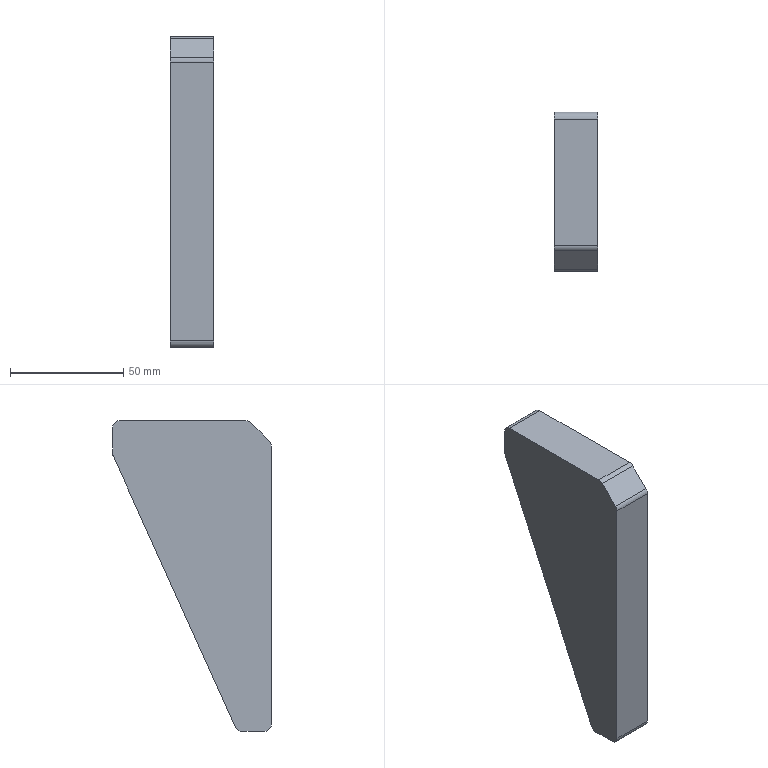Part | STEP file | SN10_010_005-03_REFORCO | 1 solid | 14 faces | box 19 x 70 x 137 mm | volume 117421 mm3 | plane 8 | cylinder 6 | commonest cylinder face diameters 6 x6
STEP:
#1=CARTESIAN_POINT('',(0.,0.,0.));
#2=DIRECTION('',(0.,0.,1.));
#3=DIRECTION('',(1.,0.,0.));
#4=AXIS2_PLACEMENT_3D('',#1,#2,#3);
#5=CARTESIAN_POINT('',(106.,-333.,340.));
#6=VERTEX_POINT('',#5);
#7=CARTESIAN_POINT('',(106.,-330.,337.));
#8=VERTEX_POINT('',#7);
#9=CARTESIAN_POINT('',(106.,-333.,337.));
#10=DIRECTION('',(-1.,0.,0.));
#11=DIRECTION('',(0.,1.,0.));
#12=AXIS2_PLACEMENT_3D('',#9,#10,#11);
#13=CIRCLE('',#12,3.);
#14=CARTESIAN_POINT('',(115.5,-333.,337.));
#15=DIRECTION('',(-1.,0.,0.));
#16=DIRECTION('',(0.,0.,1.));
#17=AXIS2_PLACEMENT_3D('',#14,#15,#16);
#18=CYLINDRICAL_SURFACE('',#17,3.);
#19=CARTESIAN_POINT('',(-4.712,9.5));
#20=DIRECTION('',(1.,0.));
#21=VECTOR('',#20,1.);
#22=LINE('',#19,#21);
#23=(GEOMETRIC_REPRESENTATION_CONTEXT(2)PARAMETRIC_REPRESENTATION_CONTEXT()REPRESENTATION_CONTEXT('',''));
#24=DEFINITIONAL_REPRESENTATION('',(#22),#23);
#25=PCURVE('',#18,#24);
#26=CARTESIAN_POINT('',(106.,0.,0.));
#27=DIRECTION('',(1.,0.,0.));
#28=DIRECTION('',(0.,0.,-1.));
#29=AXIS2_PLACEMENT_3D('',#26,#27,#28);
#30=PLANE('',#29);
#31=CARTESIAN_POINT('',(-337.,-330.));
#32=CARTESIAN_POINT('',(-331.804,-330.));
#33=CARTESIAN_POINT('',(-334.402,-334.5));
#34=CARTESIAN_POINT('',(-337.,-339.));
#35=CARTESIAN_POINT('',(-339.598,-334.5));
#36=CARTESIAN_POINT('',(-342.196,-330.));
#37=CARTESIAN_POINT('',(-337.,-330.));
#38=(BOUNDED_CURVE()B_SPLINE_CURVE(2,(#31,#32,#33,#34,#35,#36,#37),.UNSPECIFIED.,.T.,.F.)B_SPLINE_CURVE_WITH_KNOTS((1,2,2,2,2,1),(-2.094,0.,2.094,4.189,6.283,8.378),.UNSPECIFIED.)CURVE()GEOMETRIC_REPRESENTATION_ITEM()RATIONAL_B_SPLINE_CURVE((1.,0.5,1.,0.5,1.,0.5,1.))REPRESENTATION_ITEM(''));
#39=(GEOMETRIC_REPRESENTATION_CONTEXT(2)PARAMETRIC_REPRESENTATION_CONTEXT()REPRESENTATION_CONTEXT('',''));
#40=DEFINITIONAL_REPRESENTATION('',(#38),#39);
#41=PCURVE('',#30,#40);
#42=SURFACE_CURVE('',#13,(#25,#41),.PCURVE_S1.);
#43=EDGE_CURVE('',#6,#8,#42,.T.);
#44=ORIENTED_EDGE('',*,*,#43,.F.);
#45=CARTESIAN_POINT('',(125.,-333.,340.));
#46=VERTEX_POINT('',#45);
#47=CARTESIAN_POINT('',(125.,-333.,340.));
#48=DIRECTION('',(-1.,0.,0.));
#49=VECTOR('',#48,1.);
#50=LINE('',#47,#49);
#51=CARTESIAN_POINT('',(0.,-9.5));
#52=DIRECTION('',(0.,1.));
#53=VECTOR('',#52,1.);
#54=LINE('',#51,#53);
#55=(GEOMETRIC_REPRESENTATION_CONTEXT(2)PARAMETRIC_REPRESENTATION_CONTEXT()REPRESENTATION_CONTEXT('',''));
#56=DEFINITIONAL_REPRESENTATION('',(#54),#55);
#57=PCURVE('',#18,#56);
#58=CARTESIAN_POINT('',(125.,-330.,340.));
#59=DIRECTION('',(0.,0.,-1.));
#60=DIRECTION('',(-1.,0.,0.));
#61=AXIS2_PLACEMENT_3D('',#58,#59,#60);
#62=PLANE('',#61);
#63=CARTESIAN_POINT('',(0.,-3.));
#64=DIRECTION('',(1.,0.));
#65=VECTOR('',#64,1.);
#66=LINE('',#63,#65);
#67=(GEOMETRIC_REPRESENTATION_CONTEXT(2)PARAMETRIC_REPRESENTATION_CONTEXT()REPRESENTATION_CONTEXT('',''));
#68=DEFINITIONAL_REPRESENTATION('',(#66),#67);
#69=PCURVE('',#62,#68);
#70=SURFACE_CURVE('',#50,(#57,#69),.PCURVE_S1.);
#71=EDGE_CURVE('',#46,#6,#70,.T.);
#72=ORIENTED_EDGE('',*,*,#71,.F.);
#73=CARTESIAN_POINT('',(125.,-330.,337.));
#74=VERTEX_POINT('',#73);
#75=CARTESIAN_POINT('',(125.,-333.,337.));
#76=DIRECTION('',(-1.,0.,0.));
#77=DIRECTION('',(0.,1.,0.));
#78=AXIS2_PLACEMENT_3D('',#75,#76,#77);
#79=CIRCLE('',#78,3.);
#80=CARTESIAN_POINT('',(-4.712,-9.5));
#81=DIRECTION('',(1.,0.));
#82=VECTOR('',#81,1.);
#83=LINE('',#80,#82);
#84=(GEOMETRIC_REPRESENTATION_CONTEXT(2)PARAMETRIC_REPRESENTATION_CONTEXT()REPRESENTATION_CONTEXT('',''));
#85=DEFINITIONAL_REPRESENTATION('',(#83),#84);
#86=PCURVE('',#18,#85);
#87=CARTESIAN_POINT('',(125.,0.,0.));
#88=DIRECTION('',(1.,0.,0.));
#89=DIRECTION('',(0.,0.,-1.));
#90=AXIS2_PLACEMENT_3D('',#87,#88,#89);
#91=PLANE('',#90);
#92=CARTESIAN_POINT('',(-337.,-330.));
#93=CARTESIAN_POINT('',(-331.804,-330.));
#94=CARTESIAN_POINT('',(-334.402,-334.5));
#95=CARTESIAN_POINT('',(-337.,-339.));
#96=CARTESIAN_POINT('',(-339.598,-334.5));
#97=CARTESIAN_POINT('',(-342.196,-330.));
#98=CARTESIAN_POINT('',(-337.,-330.));
#99=(BOUNDED_CURVE()B_SPLINE_CURVE(2,(#92,#93,#94,#95,#96,#97,#98),.UNSPECIFIED.,.T.,.F.)B_SPLINE_CURVE_WITH_KNOTS((1,2,2,2,2,1),(-2.094,0.,2.094,4.189,6.283,8.378),.UNSPECIFIED.)CURVE()GEOMETRIC_REPRESENTATION_ITEM()RATIONAL_B_SPLINE_CURVE((1.,0.5,1.,0.5,1.,0.5,1.))REPRESENTATION_ITEM(''));
#100=(GEOMETRIC_REPRESENTATION_CONTEXT(2)PARAMETRIC_REPRESENTATION_CONTEXT()REPRESENTATION_CONTEXT('',''));
#101=DEFINITIONAL_REPRESENTATION('',(#99),#100);
#102=PCURVE('',#91,#101);
#103=SURFACE_CURVE('',#79,(#86,#102),.PCURVE_S1.);
#104=EDGE_CURVE('',#46,#74,#103,.T.);
#105=ORIENTED_EDGE('',*,*,#104,.T.);
#106=CARTESIAN_POINT('',(125.,-330.,337.));
#107=DIRECTION('',(-1.,0.,0.));
#108=VECTOR('',#107,1.);
#109=LINE('',#106,#108);
#110=CARTESIAN_POINT('',(1.571,-9.5));
#111=DIRECTION('',(0.,1.));
#112=VECTOR('',#111,1.);
#113=LINE('',#110,#112);
#114=(GEOMETRIC_REPRESENTATION_CONTEXT(2)PARAMETRIC_REPRESENTATION_CONTEXT()REPRESENTATION_CONTEXT('',''));
#115=DEFINITIONAL_REPRESENTATION('',(#113),#114);
#116=PCURVE('',#18,#115);
#117=CARTESIAN_POINT('',(125.,-330.,325.));
#118=DIRECTION('',(0.,-1.,0.));
#119=DIRECTION('',(0.,0.,-1.));
#120=AXIS2_PLACEMENT_3D('',#117,#118,#119);
#121=PLANE('',#120);
#122=CARTESIAN_POINT('',(-12.,0.));
#123=DIRECTION('',(0.,-1.));
#124=VECTOR('',#123,1.);
#125=LINE('',#122,#124);
#126=(GEOMETRIC_REPRESENTATION_CONTEXT(2)PARAMETRIC_REPRESENTATION_CONTEXT()REPRESENTATION_CONTEXT('',''));
#127=DEFINITIONAL_REPRESENTATION('',(#125),#126);
#128=PCURVE('',#121,#127);
#129=SURFACE_CURVE('',#109,(#116,#128),.PCURVE_S1.);
#130=EDGE_CURVE('',#74,#8,#129,.T.);
#131=ORIENTED_EDGE('',*,*,#130,.T.);
#132=EDGE_LOOP('',(#44,#72,#105,#131));
#133=FACE_BOUND('',#132,.T.);
#134=ADVANCED_FACE('',(#133),#18,.T.);
#135=CARTESIAN_POINT('',(125.,-330.,325.645));
#136=VERTEX_POINT('',#135);
#137=CARTESIAN_POINT('',(106.,-330.,325.645));
#138=VERTEX_POINT('',#137);
#139=CARTESIAN_POINT('',(125.,-330.,325.645));
#140=DIRECTION('',(-1.,0.,0.));
#141=VECTOR('',#140,1.);
#142=LINE('',#139,#141);
#143=CARTESIAN_POINT('',(-0.645,0.));
#144=DIRECTION('',(0.,-1.));
#145=VECTOR('',#144,1.);
#146=LINE('',#143,#145);
#147=(GEOMETRIC_REPRESENTATION_CONTEXT(2)PARAMETRIC_REPRESENTATION_CONTEXT()REPRESENTATION_CONTEXT('',''));
#148=DEFINITIONAL_REPRESENTATION('',(#146),#147);
#149=PCURVE('',#121,#148);
#150=CARTESIAN_POINT('',(115.5,-333.,325.645));
#151=DIRECTION('',(-1.,0.,0.));
#152=DIRECTION('',(0.,1.,0.));
#153=AXIS2_PLACEMENT_3D('',#150,#151,#152);
#154=CYLINDRICAL_SURFACE('',#153,3.);
#155=CARTESIAN_POINT('',(0.,-9.5));
#156=DIRECTION('',(0.,1.));
#157=VECTOR('',#156,1.);
#158=LINE('',#155,#157);
#159=(GEOMETRIC_REPRESENTATION_CONTEXT(2)PARAMETRIC_REPRESENTATION_CONTEXT()REPRESENTATION_CONTEXT('',''));
#160=DEFINITIONAL_REPRESENTATION('',(#158),#159);
#161=PCURVE('',#154,#160);
#162=SURFACE_CURVE('',#142,(#149,#161),.PCURVE_S1.);
#163=EDGE_CURVE('',#136,#138,#162,.T.);
#164=ORIENTED_EDGE('',*,*,#163,.T.);
#165=CARTESIAN_POINT('',(106.,-330.,325.645));
#166=DIRECTION('',(0.,0.,1.));
#167=VECTOR('',#166,1.);
#168=LINE('',#165,#167);
#169=CARTESIAN_POINT('',(-0.645,-19.));
#170=DIRECTION('',(-1.,0.));
#171=VECTOR('',#170,1.);
#172=LINE('',#169,#171);
#173=(GEOMETRIC_REPRESENTATION_CONTEXT(2)PARAMETRIC_REPRESENTATION_CONTEXT()REPRESENTATION_CONTEXT('',''));
#174=DEFINITIONAL_REPRESENTATION('',(#172),#173);
#175=PCURVE('',#121,#174);
#176=CARTESIAN_POINT('',(-325.645,-330.));
#177=DIRECTION('',(-1.,0.));
#178=VECTOR('',#177,1.);
#179=LINE('',#176,#178);
#180=(GEOMETRIC_REPRESENTATION_CONTEXT(2)PARAMETRIC_REPRESENTATION_CONTEXT()REPRESENTATION_CONTEXT('',''));
#181=DEFINITIONAL_REPRESENTATION('',(#179),#180);
#182=PCURVE('',#30,#181);
#183=SURFACE_CURVE('',#168,(#175,#182),.PCURVE_S1.);
#184=EDGE_CURVE('',#138,#8,#183,.T.);
#185=ORIENTED_EDGE('',*,*,#184,.T.);
#186=ORIENTED_EDGE('',*,*,#130,.F.);
#187=CARTESIAN_POINT('',(125.,-330.,325.645));
#188=DIRECTION('',(0.,0.,1.));
#189=VECTOR('',#188,1.);
#190=LINE('',#187,#189);
#191=CARTESIAN_POINT('',(-0.645,0.));
#192=DIRECTION('',(-1.,0.));
#193=VECTOR('',#192,1.);
#194=LINE('',#191,#193);
#195=(GEOMETRIC_REPRESENTATION_CONTEXT(2)PARAMETRIC_REPRESENTATION_CONTEXT()REPRESENTATION_CONTEXT('',''));
#196=DEFINITIONAL_REPRESENTATION('',(#194),#195);
#197=PCURVE('',#121,#196);
#198=CARTESIAN_POINT('',(-325.645,-330.));
#199=DIRECTION('',(-1.,0.));
#200=VECTOR('',#199,1.);
#201=LINE('',#198,#200);
#202=(GEOMETRIC_REPRESENTATION_CONTEXT(2)PARAMETRIC_REPRESENTATION_CONTEXT()REPRESENTATION_CONTEXT('',''));
#203=DEFINITIONAL_REPRESENTATION('',(#201),#202);
#204=PCURVE('',#91,#203);
#205=SURFACE_CURVE('',#190,(#197,#204),.PCURVE_S1.);
#206=EDGE_CURVE('',#136,#74,#205,.T.);
#207=ORIENTED_EDGE('',*,*,#206,.F.);
#208=EDGE_LOOP('',(#164,#185,#186,#207));
#209=FACE_BOUND('',#208,.T.);
#210=ADVANCED_FACE('',(#209),#121,.F.);
#211=CARTESIAN_POINT('',(106.,-330.265,324.412));
#212=VERTEX_POINT('',#211);
#213=CARTESIAN_POINT('',(106.,-333.,325.645));
#214=DIRECTION('',(-1.,0.,0.));
#215=DIRECTION('',(0.,1.,0.));
#216=AXIS2_PLACEMENT_3D('',#213,#214,#215);
#217=CIRCLE('',#216,3.);
#218=CARTESIAN_POINT('',(0.,9.5));
#219=DIRECTION('',(1.,0.));
#220=VECTOR('',#219,1.);
#221=LINE('',#218,#220);
#222=(GEOMETRIC_REPRESENTATION_CONTEXT(2)PARAMETRIC_REPRESENTATION_CONTEXT()REPRESENTATION_CONTEXT('',''));
#223=DEFINITIONAL_REPRESENTATION('',(#221),#222);
#224=PCURVE('',#154,#223);
#225=CARTESIAN_POINT('',(-325.645,-330.));
#226=CARTESIAN_POINT('',(-320.449,-330.));
#227=CARTESIAN_POINT('',(-323.047,-334.5));
#228=CARTESIAN_POINT('',(-325.645,-339.));
#229=CARTESIAN_POINT('',(-328.243,-334.5));
#230=CARTESIAN_POINT('',(-330.841,-330.));
#231=CARTESIAN_POINT('',(-325.645,-330.));
#232=(BOUNDED_CURVE()B_SPLINE_CURVE(2,(#225,#226,#227,#228,#229,#230,#231),.UNSPECIFIED.,.T.,.F.)B_SPLINE_CURVE_WITH_KNOTS((1,2,2,2,2,1),(-2.094,0.,2.094,4.189,6.283,8.378),.UNSPECIFIED.)CURVE()GEOMETRIC_REPRESENTATION_ITEM()RATIONAL_B_SPLINE_CURVE((1.,0.5,1.,0.5,1.,0.5,1.))REPRESENTATION_ITEM(''));
#233=(GEOMETRIC_REPRESENTATION_CONTEXT(2)PARAMETRIC_REPRESENTATION_CONTEXT()REPRESENTATION_CONTEXT('',''));
#234=DEFINITIONAL_REPRESENTATION('',(#232),#233);
#235=PCURVE('',#30,#234);
#236=SURFACE_CURVE('',#217,(#224,#235),.PCURVE_S1.);
#237=EDGE_CURVE('',#138,#212,#236,.T.);
#238=ORIENTED_EDGE('',*,*,#237,.F.);
#239=ORIENTED_EDGE('',*,*,#163,.F.);
#240=CARTESIAN_POINT('',(125.,-330.265,324.412));
#241=VERTEX_POINT('',#240);
#242=CARTESIAN_POINT('',(125.,-333.,325.645));
#243=DIRECTION('',(-1.,0.,0.));
#244=DIRECTION('',(0.,1.,0.));
#245=AXIS2_PLACEMENT_3D('',#242,#243,#244);
#246=CIRCLE('',#245,3.);
#247=CARTESIAN_POINT('',(0.,-9.5));
#248=DIRECTION('',(1.,0.));
#249=VECTOR('',#248,1.);
#250=LINE('',#247,#249);
#251=(GEOMETRIC_REPRESENTATION_CONTEXT(2)PARAMETRIC_REPRESENTATION_CONTEXT()REPRESENTATION_CONTEXT('',''));
#252=DEFINITIONAL_REPRESENTATION('',(#250),#251);
#253=PCURVE('',#154,#252);
#254=CARTESIAN_POINT('',(-325.645,-330.));
#255=CARTESIAN_POINT('',(-320.449,-330.));
#256=CARTESIAN_POINT('',(-323.047,-334.5));
#257=CARTESIAN_POINT('',(-325.645,-339.));
#258=CARTESIAN_POINT('',(-328.243,-334.5));
#259=CARTESIAN_POINT('',(-330.841,-330.));
#260=CARTESIAN_POINT('',(-325.645,-330.));
#261=(BOUNDED_CURVE()B_SPLINE_CURVE(2,(#254,#255,#256,#257,#258,#259,#260),.UNSPECIFIED.,.T.,.F.)B_SPLINE_CURVE_WITH_KNOTS((1,2,2,2,2,1),(-2.094,0.,2.094,4.189,6.283,8.378),.UNSPECIFIED.)CURVE()GEOMETRIC_REPRESENTATION_ITEM()RATIONAL_B_SPLINE_CURVE((1.,0.5,1.,0.5,1.,0.5,1.))REPRESENTATION_ITEM(''));
#262=(GEOMETRIC_REPRESENTATION_CONTEXT(2)PARAMETRIC_REPRESENTATION_CONTEXT()REPRESENTATION_CONTEXT('',''));
#263=DEFINITIONAL_REPRESENTATION('',(#261),#262);
#264=PCURVE('',#91,#263);
#265=SURFACE_CURVE('',#246,(#253,#264),.PCURVE_S1.);
#266=EDGE_CURVE('',#136,#241,#265,.T.);
#267=ORIENTED_EDGE('',*,*,#266,.T.);
#268=CARTESIAN_POINT('',(125.,-330.265,324.412));
#269=DIRECTION('',(-1.,0.,0.));
#270=VECTOR('',#269,1.);
#271=LINE('',#268,#270);
#272=CARTESIAN_POINT('',(0.4235,-9.5));
#273=DIRECTION('',(0.,1.));
#274=VECTOR('',#273,1.);
#275=LINE('',#272,#274);
#276=(GEOMETRIC_REPRESENTATION_CONTEXT(2)PARAMETRIC_REPRESENTATION_CONTEXT()REPRESENTATION_CONTEXT('',''));
#277=DEFINITIONAL_REPRESENTATION('',(#275),#276);
#278=PCURVE('',#154,#277);
#279=CARTESIAN_POINT('',(125.,-385.,203.));
#280=DIRECTION('',(0.,-0.9116,0.411));
#281=DIRECTION('',(0.,-0.411,-0.9116));
#282=AXIS2_PLACEMENT_3D('',#279,#280,#281);
#283=PLANE('',#282);
#284=CARTESIAN_POINT('',(-133.18,0.));
#285=DIRECTION('',(0.,-1.));
#286=VECTOR('',#285,1.);
#287=LINE('',#284,#286);
#288=(GEOMETRIC_REPRESENTATION_CONTEXT(2)PARAMETRIC_REPRESENTATION_CONTEXT()REPRESENTATION_CONTEXT('',''));
#289=DEFINITIONAL_REPRESENTATION('',(#287),#288);
#290=PCURVE('',#283,#289);
#291=SURFACE_CURVE('',#271,(#278,#290),.PCURVE_S1.);
#292=EDGE_CURVE('',#241,#212,#291,.T.);
#293=ORIENTED_EDGE('',*,*,#292,.T.);
#294=EDGE_LOOP('',(#238,#239,#267,#293));
#295=FACE_BOUND('',#294,.T.);
#296=ADVANCED_FACE('',(#295),#154,.T.);
#297=CARTESIAN_POINT('',(125.,-384.203,204.767));
#298=VERTEX_POINT('',#297);
#299=CARTESIAN_POINT('',(106.,-384.203,204.767));
#300=VERTEX_POINT('',#299);
#301=CARTESIAN_POINT('',(125.,-384.203,204.767));
#302=DIRECTION('',(-1.,0.,0.));
#303=VECTOR('',#302,1.);
#304=LINE('',#301,#303);
#305=CARTESIAN_POINT('',(-1.938,0.));
#306=DIRECTION('',(0.,-1.));
#307=VECTOR('',#306,1.);
#308=LINE('',#305,#307);
#309=(GEOMETRIC_REPRESENTATION_CONTEXT(2)PARAMETRIC_REPRESENTATION_CONTEXT()REPRESENTATION_CONTEXT('',''));
#310=DEFINITIONAL_REPRESENTATION('',(#308),#309);
#311=PCURVE('',#283,#310);
#312=CARTESIAN_POINT('',(115.5,-386.938,206.));
#313=DIRECTION('',(-1.,0.,0.));
#314=DIRECTION('',(0.,0.9116,-0.411));
#315=AXIS2_PLACEMENT_3D('',#312,#313,#314);
#316=CYLINDRICAL_SURFACE('',#315,3.);
#317=CARTESIAN_POINT('',(0.,-9.5));
#318=DIRECTION('',(0.,1.));
#319=VECTOR('',#318,1.);
#320=LINE('',#317,#319);
#321=(GEOMETRIC_REPRESENTATION_CONTEXT(2)PARAMETRIC_REPRESENTATION_CONTEXT()REPRESENTATION_CONTEXT('',''));
#322=DEFINITIONAL_REPRESENTATION('',(#320),#321);
#323=PCURVE('',#316,#322);
#324=SURFACE_CURVE('',#304,(#311,#323),.PCURVE_S1.);
#325=EDGE_CURVE('',#298,#300,#324,.T.);
#326=ORIENTED_EDGE('',*,*,#325,.T.);
#327=CARTESIAN_POINT('',(106.,-384.203,204.767));
#328=DIRECTION('',(0.,0.411,0.9116));
#329=VECTOR('',#328,1.);
#330=LINE('',#327,#329);
#331=CARTESIAN_POINT('',(-1.938,-19.));
#332=DIRECTION('',(-1.,0.));
#333=VECTOR('',#332,1.);
#334=LINE('',#331,#333);
#335=(GEOMETRIC_REPRESENTATION_CONTEXT(2)PARAMETRIC_REPRESENTATION_CONTEXT()REPRESENTATION_CONTEXT('',''));
#336=DEFINITIONAL_REPRESENTATION('',(#334),#335);
#337=PCURVE('',#283,#336);
#338=CARTESIAN_POINT('',(-204.767,-384.203));
#339=DIRECTION('',(-0.9116,0.411));
#340=VECTOR('',#339,1.);
#341=LINE('',#338,#340);
#342=(GEOMETRIC_REPRESENTATION_CONTEXT(2)PARAMETRIC_REPRESENTATION_CONTEXT()REPRESENTATION_CONTEXT('',''));
#343=DEFINITIONAL_REPRESENTATION('',(#341),#342);
#344=PCURVE('',#30,#343);
#345=SURFACE_CURVE('',#330,(#337,#344),.PCURVE_S1.);
#346=EDGE_CURVE('',#300,#212,#345,.T.);
#347=ORIENTED_EDGE('',*,*,#346,.T.);
#348=ORIENTED_EDGE('',*,*,#292,.F.);
#349=CARTESIAN_POINT('',(125.,-384.203,204.767));
#350=DIRECTION('',(0.,0.411,0.9116));
#351=VECTOR('',#350,1.);
#352=LINE('',#349,#351);
#353=CARTESIAN_POINT('',(-1.938,0.));
#354=DIRECTION('',(-1.,0.));
#355=VECTOR('',#354,1.);
#356=LINE('',#353,#355);
#357=(GEOMETRIC_REPRESENTATION_CONTEXT(2)PARAMETRIC_REPRESENTATION_CONTEXT()REPRESENTATION_CONTEXT('',''));
#358=DEFINITIONAL_REPRESENTATION('',(#356),#357);
#359=PCURVE('',#283,#358);
#360=CARTESIAN_POINT('',(-204.767,-384.203));
#361=DIRECTION('',(-0.9116,0.411));
#362=VECTOR('',#361,1.);
#363=LINE('',#360,#362);
#364=(GEOMETRIC_REPRESENTATION_CONTEXT(2)PARAMETRIC_REPRESENTATION_CONTEXT()REPRESENTATION_CONTEXT('',''));
#365=DEFINITIONAL_REPRESENTATION('',(#363),#364);
#366=PCURVE('',#91,#365);
#367=SURFACE_CURVE('',#352,(#359,#366),.PCURVE_S1.);
#368=EDGE_CURVE('',#298,#241,#367,.T.);
#369=ORIENTED_EDGE('',*,*,#368,.F.);
#370=EDGE_LOOP('',(#326,#347,#348,#369));
#371=FACE_BOUND('',#370,.T.);
#372=ADVANCED_FACE('',(#371),#283,.F.);
#373=CARTESIAN_POINT('',(106.,-386.938,203.));
#374=VERTEX_POINT('',#373);
#375=CARTESIAN_POINT('',(106.,-386.938,206.));
#376=DIRECTION('',(-1.,0.,0.));
#377=DIRECTION('',(0.,1.,0.));
#378=AXIS2_PLACEMENT_3D('',#375,#376,#377);
#379=CIRCLE('',#378,3.);
#380=CARTESIAN_POINT('',(-0.4235,9.5));
#381=DIRECTION('',(1.,0.));
#382=VECTOR('',#381,1.);
#383=LINE('',#380,#382);
#384=(GEOMETRIC_REPRESENTATION_CONTEXT(2)PARAMETRIC_REPRESENTATION_CONTEXT()REPRESENTATION_CONTEXT('',''));
#385=DEFINITIONAL_REPRESENTATION('',(#383),#384);
#386=PCURVE('',#316,#385);
#387=CARTESIAN_POINT('',(-206.,-383.938));
#388=CARTESIAN_POINT('',(-200.804,-383.938));
#389=CARTESIAN_POINT('',(-203.402,-388.438));
#390=CARTESIAN_POINT('',(-206.,-392.938));
#391=CARTESIAN_POINT('',(-208.598,-388.438));
#392=CARTESIAN_POINT('',(-211.196,-383.938));
#393=CARTESIAN_POINT('',(-206.,-383.938));
#394=(BOUNDED_CURVE()B_SPLINE_CURVE(2,(#387,#388,#389,#390,#391,#392,#393),.UNSPECIFIED.,.T.,.F.)B_SPLINE_CURVE_WITH_KNOTS((1,2,2,2,2,1),(-2.094,0.,2.094,4.189,6.283,8.378),.UNSPECIFIED.)CURVE()GEOMETRIC_REPRESENTATION_ITEM()RATIONAL_B_SPLINE_CURVE((1.,0.5,1.,0.5,1.,0.5,1.))REPRESENTATION_ITEM(''));
#395=(GEOMETRIC_REPRESENTATION_CONTEXT(2)PARAMETRIC_REPRESENTATION_CONTEXT()REPRESENTATION_CONTEXT('',''));
#396=DEFINITIONAL_REPRESENTATION('',(#394),#395);
#397=PCURVE('',#30,#396);
#398=SURFACE_CURVE('',#379,(#386,#397),.PCURVE_S1.);
#399=EDGE_CURVE('',#300,#374,#398,.T.);
#400=ORIENTED_EDGE('',*,*,#399,.F.);
#401=ORIENTED_EDGE('',*,*,#325,.F.);
#402=CARTESIAN_POINT('',(125.,-386.938,203.));
#403=VERTEX_POINT('',#402);
#404=CARTESIAN_POINT('',(125.,-386.938,206.));
#405=DIRECTION('',(-1.,0.,0.));
#406=DIRECTION('',(0.,1.,0.));
#407=AXIS2_PLACEMENT_3D('',#404,#405,#406);
#408=CIRCLE('',#407,3.);
#409=CARTESIAN_POINT('',(-0.4235,-9.5));
#410=DIRECTION('',(1.,0.));
#411=VECTOR('',#410,1.);
#412=LINE('',#409,#411);
#413=(GEOMETRIC_REPRESENTATION_CONTEXT(2)PARAMETRIC_REPRESENTATION_CONTEXT()REPRESENTATION_CONTEXT('',''));
#414=DEFINITIONAL_REPRESENTATION('',(#412),#413);
#415=PCURVE('',#316,#414);
#416=CARTESIAN_POINT('',(-206.,-383.938));
#417=CARTESIAN_POINT('',(-200.804,-383.938));
#418=CARTESIAN_POINT('',(-203.402,-388.438));
#419=CARTESIAN_POINT('',(-206.,-392.938));
#420=CARTESIAN_POINT('',(-208.598,-388.438));
#421=CARTESIAN_POINT('',(-211.196,-383.938));
#422=CARTESIAN_POINT('',(-206.,-383.938));
#423=(BOUNDED_CURVE()B_SPLINE_CURVE(2,(#416,#417,#418,#419,#420,#421,#422),.UNSPECIFIED.,.T.,.F.)B_SPLINE_CURVE_WITH_KNOTS((1,2,2,2,2,1),(-2.094,0.,2.094,4.189,6.283,8.378),.UNSPECIFIED.)CURVE()GEOMETRIC_REPRESENTATION_ITEM()RATIONAL_B_SPLINE_CURVE((1.,0.5,1.,0.5,1.,0.5,1.))REPRESENTATION_ITEM(''));
#424=(GEOMETRIC_REPRESENTATION_CONTEXT(2)PARAMETRIC_REPRESENTATION_CONTEXT()REPRESENTATION_CONTEXT('',''));
#425=DEFINITIONAL_REPRESENTATION('',(#423),#424);
#426=PCURVE('',#91,#425);
#427=SURFACE_CURVE('',#408,(#415,#426),.PCURVE_S1.);
#428=EDGE_CURVE('',#298,#403,#427,.T.);
#429=ORIENTED_EDGE('',*,*,#428,.T.);
#430=CARTESIAN_POINT('',(125.,-386.938,203.));
#431=DIRECTION('',(-1.,0.,0.));
#432=VECTOR('',#431,1.);
#433=LINE('',#430,#432);
#434=CARTESIAN_POINT('',(1.147,-9.5));
#435=DIRECTION('',(0.,1.));
#436=VECTOR('',#435,1.);
#437=LINE('',#434,#436);
#438=(GEOMETRIC_REPRESENTATION_CONTEXT(2)PARAMETRIC_REPRESENTATION_CONTEXT()REPRESENTATION_CONTEXT('',''));
#439=DEFINITIONAL_REPRESENTATION('',(#437),#438);
#440=PCURVE('',#316,#439);
#441=CARTESIAN_POINT('',(125.,-400.,203.));
#442=DIRECTION('',(0.,0.,1.));
#443=DIRECTION('',(1.,0.,0.));
#444=AXIS2_PLACEMENT_3D('',#441,#442,#443);
#445=PLANE('',#444);
#446=CARTESIAN_POINT('',(0.,13.062));
#447=DIRECTION('',(-1.,0.));
#448=VECTOR('',#447,1.);
#449=LINE('',#446,#448);
#450=(GEOMETRIC_REPRESENTATION_CONTEXT(2)PARAMETRIC_REPRESENTATION_CONTEXT()REPRESENTATION_CONTEXT('',''));
#451=DEFINITIONAL_REPRESENTATION('',(#449),#450);
#452=PCURVE('',#445,#451);
#453=SURFACE_CURVE('',#433,(#440,#452),.PCURVE_S1.);
#454=EDGE_CURVE('',#403,#374,#453,.T.);
#455=ORIENTED_EDGE('',*,*,#454,.T.);
#456=EDGE_LOOP('',(#400,#401,#429,#455));
#457=FACE_BOUND('',#456,.T.);
#458=ADVANCED_FACE('',(#457),#316,.T.);
#459=CARTESIAN_POINT('',(125.,-397.,203.));
#460=VERTEX_POINT('',#459);
#461=CARTESIAN_POINT('',(106.,-397.,203.));
#462=VERTEX_POINT('',#461);
#463=CARTESIAN_POINT('',(125.,-397.,203.));
#464=DIRECTION('',(-1.,0.,0.));
#465=VECTOR('',#464,1.);
#466=LINE('',#463,#465);
#467=CARTESIAN_POINT('',(0.,3.));
#468=DIRECTION('',(-1.,0.));
#469=VECTOR('',#468,1.);
#470=LINE('',#467,#469);
#471=(GEOMETRIC_REPRESENTATION_CONTEXT(2)PARAMETRIC_REPRESENTATION_CONTEXT()REPRESENTATION_CONTEXT('',''));
#472=DEFINITIONAL_REPRESENTATION('',(#470),#471);
#473=PCURVE('',#445,#472);
#474=CARTESIAN_POINT('',(115.5,-397.,206.));
#475=DIRECTION('',(-1.,0.,0.));
#476=DIRECTION('',(0.,0.,-1.));
#477=AXIS2_PLACEMENT_3D('',#474,#475,#476);
#478=CYLINDRICAL_SURFACE('',#477,3.);
#479=CARTESIAN_POINT('',(0.,-9.5));
#480=DIRECTION('',(0.,1.));
#481=VECTOR('',#480,1.);
#482=LINE('',#479,#481);
#483=(GEOMETRIC_REPRESENTATION_CONTEXT(2)PARAMETRIC_REPRESENTATION_CONTEXT()REPRESENTATION_CONTEXT('',''));
#484=DEFINITIONAL_REPRESENTATION('',(#482),#483);
#485=PCURVE('',#478,#484);
#486=SURFACE_CURVE('',#466,(#473,#485),.PCURVE_S1.);
#487=EDGE_CURVE('',#460,#462,#486,.T.);
#488=ORIENTED_EDGE('',*,*,#487,.T.);
#489=CARTESIAN_POINT('',(106.,-397.,203.));
#490=DIRECTION('',(0.,1.,0.));
#491=VECTOR('',#490,1.);
#492=LINE('',#489,#491);
#493=CARTESIAN_POINT('',(-19.,3.));
#494=DIRECTION('',(0.,1.));
#495=VECTOR('',#494,1.);
#496=LINE('',#493,#495);
#497=(GEOMETRIC_REPRESENTATION_CONTEXT(2)PARAMETRIC_REPRESENTATION_CONTEXT()REPRESENTATION_CONTEXT('',''));
#498=DEFINITIONAL_REPRESENTATION('',(#496),#497);
#499=PCURVE('',#445,#498);
#500=CARTESIAN_POINT('',(-203.,-397.));
#501=DIRECTION('',(0.,1.));
#502=VECTOR('',#501,1.);
#503=LINE('',#500,#502);
#504=(GEOMETRIC_REPRESENTATION_CONTEXT(2)PARAMETRIC_REPRESENTATION_CONTEXT()REPRESENTATION_CONTEXT('',''));
#505=DEFINITIONAL_REPRESENTATION('',(#503),#504);
#506=PCURVE('',#30,#505);
#507=SURFACE_CURVE('',#492,(#499,#506),.PCURVE_S1.);
#508=EDGE_CURVE('',#462,#374,#507,.T.);
#509=ORIENTED_EDGE('',*,*,#508,.T.);
#510=ORIENTED_EDGE('',*,*,#454,.F.);
#511=CARTESIAN_POINT('',(125.,-397.,203.));
#512=DIRECTION('',(0.,1.,0.));
#513=VECTOR('',#512,1.);
#514=LINE('',#511,#513);
#515=CARTESIAN_POINT('',(0.,3.));
#516=DIRECTION('',(0.,1.));
#517=VECTOR('',#516,1.);
#518=LINE('',#515,#517);
#519=(GEOMETRIC_REPRESENTATION_CONTEXT(2)PARAMETRIC_REPRESENTATION_CONTEXT()REPRESENTATION_CONTEXT('',''));
#520=DEFINITIONAL_REPRESENTATION('',(#518),#519);
#521=PCURVE('',#445,#520);
#522=CARTESIAN_POINT('',(-203.,-397.));
#523=DIRECTION('',(0.,1.));
#524=VECTOR('',#523,1.);
#525=LINE('',#522,#524);
#526=(GEOMETRIC_REPRESENTATION_CONTEXT(2)PARAMETRIC_REPRESENTATION_CONTEXT()REPRESENTATION_CONTEXT('',''));
#527=DEFINITIONAL_REPRESENTATION('',(#525),#526);
#528=PCURVE('',#91,#527);
#529=SURFACE_CURVE('',#514,(#521,#528),.PCURVE_S1.);
#530=EDGE_CURVE('',#460,#403,#529,.T.);
#531=ORIENTED_EDGE('',*,*,#530,.F.);
#532=EDGE_LOOP('',(#488,#509,#510,#531));
#533=FACE_BOUND('',#532,.T.);
#534=ADVANCED_FACE('',(#533),#445,.F.);
#535=CARTESIAN_POINT('',(106.,-400.,206.));
#536=VERTEX_POINT('',#535);
#537=CARTESIAN_POINT('',(106.,-397.,206.));
#538=DIRECTION('',(-1.,0.,0.));
#539=DIRECTION('',(0.,1.,0.));
#540=AXIS2_PLACEMENT_3D('',#537,#538,#539);
#541=CIRCLE('',#540,3.);
#542=CARTESIAN_POINT('',(-1.571,9.5));
#543=DIRECTION('',(1.,0.));
#544=VECTOR('',#543,1.);
#545=LINE('',#542,#544);
#546=(GEOMETRIC_REPRESENTATION_CONTEXT(2)PARAMETRIC_REPRESENTATION_CONTEXT()REPRESENTATION_CONTEXT('',''));
#547=DEFINITIONAL_REPRESENTATION('',(#545),#546);
#548=PCURVE('',#478,#547);
#549=CARTESIAN_POINT('',(-206.,-394.));
#550=CARTESIAN_POINT('',(-200.804,-394.));
#551=CARTESIAN_POINT('',(-203.402,-398.5));
#552=CARTESIAN_POINT('',(-206.,-403.));
#553=CARTESIAN_POINT('',(-208.598,-398.5));
#554=CARTESIAN_POINT('',(-211.196,-394.));
#555=CARTESIAN_POINT('',(-206.,-394.));
#556=(BOUNDED_CURVE()B_SPLINE_CURVE(2,(#549,#550,#551,#552,#553,#554,#555),.UNSPECIFIED.,.T.,.F.)B_SPLINE_CURVE_WITH_KNOTS((1,2,2,2,2,1),(-2.094,0.,2.094,4.189,6.283,8.378),.UNSPECIFIED.)CURVE()GEOMETRIC_REPRESENTATION_ITEM()RATIONAL_B_SPLINE_CURVE((1.,0.5,1.,0.5,1.,0.5,1.))REPRESENTATION_ITEM(''));
#557=(GEOMETRIC_REPRESENTATION_CONTEXT(2)PARAMETRIC_REPRESENTATION_CONTEXT()REPRESENTATION_CONTEXT('',''));
#558=DEFINITIONAL_REPRESENTATION('',(#556),#557);
#559=PCURVE('',#30,#558);
#560=SURFACE_CURVE('',#541,(#548,#559),.PCURVE_S1.);
#561=EDGE_CURVE('',#462,#536,#560,.T.);
#562=ORIENTED_EDGE('',*,*,#561,.F.);
#563=ORIENTED_EDGE('',*,*,#487,.F.);
#564=CARTESIAN_POINT('',(125.,-400.,206.));
#565=VERTEX_POINT('',#564);
#566=CARTESIAN_POINT('',(125.,-397.,206.));
#567=DIRECTION('',(-1.,0.,0.));
#568=DIRECTION('',(0.,1.,0.));
#569=AXIS2_PLACEMENT_3D('',#566,#567,#568);
#570=CIRCLE('',#569,3.);
#571=CARTESIAN_POINT('',(-1.571,-9.5));
#572=DIRECTION('',(1.,0.));
#573=VECTOR('',#572,1.);
#574=LINE('',#571,#573);
#575=(GEOMETRIC_REPRESENTATION_CONTEXT(2)PARAMETRIC_REPRESENTATION_CONTEXT()REPRESENTATION_CONTEXT('',''));
#576=DEFINITIONAL_REPRESENTATION('',(#574),#575);
#577=PCURVE('',#478,#576);
#578=CARTESIAN_POINT('',(-206.,-394.));
#579=CARTESIAN_POINT('',(-200.804,-394.));
#580=CARTESIAN_POINT('',(-203.402,-398.5));
#581=CARTESIAN_POINT('',(-206.,-403.));
#582=CARTESIAN_POINT('',(-208.598,-398.5));
#583=CARTESIAN_POINT('',(-211.196,-394.));
#584=CARTESIAN_POINT('',(-206.,-394.));
#585=(BOUNDED_CURVE()B_SPLINE_CURVE(2,(#578,#579,#580,#581,#582,#583,#584),.UNSPECIFIED.,.T.,.F.)B_SPLINE_CURVE_WITH_KNOTS((1,2,2,2,2,1),(-2.094,0.,2.094,4.189,6.283,8.378),.UNSPECIFIED.)CURVE()GEOMETRIC_REPRESENTATION_ITEM()RATIONAL_B_SPLINE_CURVE((1.,0.5,1.,0.5,1.,0.5,1.))REPRESENTATION_ITEM(''));
#586=(GEOMETRIC_REPRESENTATION_CONTEXT(2)PARAMETRIC_REPRESENTATION_CONTEXT()REPRESENTATION_CONTEXT('',''));
#587=DEFINITIONAL_REPRESENTATION('',(#585),#586);
#588=PCURVE('',#91,#587);
#589=SURFACE_CURVE('',#570,(#577,#588),.PCURVE_S1.);
#590=EDGE_CURVE('',#460,#565,#589,.T.);
#591=ORIENTED_EDGE('',*,*,#590,.T.);
#592=CARTESIAN_POINT('',(125.,-400.,206.));
#593=DIRECTION('',(-1.,0.,0.));
#594=VECTOR('',#593,1.);
#595=LINE('',#592,#594);
#596=CARTESIAN_POINT('',(1.571,-9.5));
#597=DIRECTION('',(0.,1.));
#598=VECTOR('',#597,1.);
#599=LINE('',#596,#598);
#600=(GEOMETRIC_REPRESENTATION_CONTEXT(2)PARAMETRIC_REPRESENTATION_CONTEXT()REPRESENTATION_CONTEXT('',''));
#601=DEFINITIONAL_REPRESENTATION('',(#599),#600);
#602=PCURVE('',#478,#601);
#603=CARTESIAN_POINT('',(125.,-400.,330.));
#604=DIRECTION('',(0.,1.,0.));
#605=DIRECTION('',(0.,0.,1.));
#606=AXIS2_PLACEMENT_3D('',#603,#604,#605);
#607=PLANE('',#606);
#608=CARTESIAN_POINT('',(-124.,0.));
#609=DIRECTION('',(0.,-1.));
#610=VECTOR('',#609,1.);
#611=LINE('',#608,#610);
#612=(GEOMETRIC_REPRESENTATION_CONTEXT(2)PARAMETRIC_REPRESENTATION_CONTEXT()REPRESENTATION_CONTEXT('',''));
#613=DEFINITIONAL_REPRESENTATION('',(#611),#612);
#614=PCURVE('',#607,#613);
#615=SURFACE_CURVE('',#595,(#602,#614),.PCURVE_S1.);
#616=EDGE_CURVE('',#565,#536,#615,.T.);
#617=ORIENTED_EDGE('',*,*,#616,.T.);
#618=EDGE_LOOP('',(#562,#563,#591,#617));
#619=FACE_BOUND('',#618,.T.);
#620=ADVANCED_FACE('',(#619),#478,.T.);
#621=CARTESIAN_POINT('',(125.,-400.,328.757));
#622=VERTEX_POINT('',#621);
#623=CARTESIAN_POINT('',(106.,-400.,328.757));
#624=VERTEX_POINT('',#623);
#625=CARTESIAN_POINT('',(125.,-400.,328.757));
#626=DIRECTION('',(-1.,0.,0.));
#627=VECTOR('',#626,1.);
#628=LINE('',#625,#627);
#629=CARTESIAN_POINT('',(-1.243,0.));
#630=DIRECTION('',(0.,-1.));
#631=VECTOR('',#630,1.);
#632=LINE('',#629,#631);
#633=(GEOMETRIC_REPRESENTATION_CONTEXT(2)PARAMETRIC_REPRESENTATION_CONTEXT()REPRESENTATION_CONTEXT('',''));
#634=DEFINITIONAL_REPRESENTATION('',(#632),#633);
#635=PCURVE('',#607,#634);
#636=CARTESIAN_POINT('',(115.5,-397.,328.757));
#637=DIRECTION('',(-1.,0.,0.));
#638=DIRECTION('',(0.,-1.,0.));
#639=AXIS2_PLACEMENT_3D('',#636,#637,#638);
#640=CYLINDRICAL_SURFACE('',#639,3.);
#641=CARTESIAN_POINT('',(0.,-9.5));
#642=DIRECTION('',(0.,1.));
#643=VECTOR('',#642,1.);
#644=LINE('',#641,#643);
#645=(GEOMETRIC_REPRESENTATION_CONTEXT(2)PARAMETRIC_REPRESENTATION_CONTEXT()REPRESENTATION_CONTEXT('',''));
#646=DEFINITIONAL_REPRESENTATION('',(#644),#645);
#647=PCURVE('',#640,#646);
#648=SURFACE_CURVE('',#628,(#635,#647),.PCURVE_S1.);
#649=EDGE_CURVE('',#622,#624,#648,.T.);
#650=ORIENTED_EDGE('',*,*,#649,.T.);
#651=CARTESIAN_POINT('',(106.,-400.,328.757));
#652=DIRECTION('',(0.,0.,-1.));
#653=VECTOR('',#652,1.);
#654=LINE('',#651,#653);
#655=CARTESIAN_POINT('',(-1.243,-19.));
#656=DIRECTION('',(-1.,0.));
#657=VECTOR('',#656,1.);
#658=LINE('',#655,#657);
#659=(GEOMETRIC_REPRESENTATION_CONTEXT(2)PARAMETRIC_REPRESENTATION_CONTEXT()REPRESENTATION_CONTEXT('',''));
#660=DEFINITIONAL_REPRESENTATION('',(#658),#659);
#661=PCURVE('',#607,#660);
#662=CARTESIAN_POINT('',(-328.757,-400.));
#663=DIRECTION('',(1.,0.));
#664=VECTOR('',#663,1.);
#665=LINE('',#662,#664);
#666=(GEOMETRIC_REPRESENTATION_CONTEXT(2)PARAMETRIC_REPRESENTATION_CONTEXT()REPRESENTATION_CONTEXT('',''));
#667=DEFINITIONAL_REPRESENTATION('',(#665),#666);
#668=PCURVE('',#30,#667);
#669=SURFACE_CURVE('',#654,(#661,#668),.PCURVE_S1.);
#670=EDGE_CURVE('',#624,#536,#669,.T.);
#671=ORIENTED_EDGE('',*,*,#670,.T.);
#672=ORIENTED_EDGE('',*,*,#616,.F.);
#673=CARTESIAN_POINT('',(125.,-400.,328.757));
#674=DIRECTION('',(0.,0.,-1.));
#675=VECTOR('',#674,1.);
#676=LINE('',#673,#675);
#677=CARTESIAN_POINT('',(-1.243,0.));
#678=DIRECTION('',(-1.,0.));
#679=VECTOR('',#678,1.);
#680=LINE('',#677,#679);
#681=(GEOMETRIC_REPRESENTATION_CONTEXT(2)PARAMETRIC_REPRESENTATION_CONTEXT()REPRESENTATION_CONTEXT('',''));
#682=DEFINITIONAL_REPRESENTATION('',(#680),#681);
#683=PCURVE('',#607,#682);
#684=CARTESIAN_POINT('',(-328.757,-400.));
#685=DIRECTION('',(1.,0.));
#686=VECTOR('',#685,1.);
#687=LINE('',#684,#686);
#688=(GEOMETRIC_REPRESENTATION_CONTEXT(2)PARAMETRIC_REPRESENTATION_CONTEXT()REPRESENTATION_CONTEXT('',''));
#689=DEFINITIONAL_REPRESENTATION('',(#687),#688);
#690=PCURVE('',#91,#689);
#691=SURFACE_CURVE('',#676,(#683,#690),.PCURVE_S1.);
#692=EDGE_CURVE('',#622,#565,#691,.T.);
#693=ORIENTED_EDGE('',*,*,#692,.F.);
#694=EDGE_LOOP('',(#650,#671,#672,#693));
#695=FACE_BOUND('',#694,.T.);
#696=ADVANCED_FACE('',(#695),#607,.F.);
#697=CARTESIAN_POINT('',(106.,-399.121,330.879));
#698=VERTEX_POINT('',#697);
#699=CARTESIAN_POINT('',(106.,-397.,328.757));
#700=DIRECTION('',(-1.,0.,0.));
#701=DIRECTION('',(0.,1.,0.));
#702=AXIS2_PLACEMENT_3D('',#699,#700,#701);
#703=CIRCLE('',#702,3.);
#704=CARTESIAN_POINT('',(-3.142,9.5));
#705=DIRECTION('',(1.,0.));
#706=VECTOR('',#705,1.);
#707=LINE('',#704,#706);
#708=(GEOMETRIC_REPRESENTATION_CONTEXT(2)PARAMETRIC_REPRESENTATION_CONTEXT()REPRESENTATION_CONTEXT('',''));
#709=DEFINITIONAL_REPRESENTATION('',(#707),#708);
#710=PCURVE('',#640,#709);
#711=CARTESIAN_POINT('',(-328.757,-394.));
#712=CARTESIAN_POINT('',(-323.561,-394.));
#713=CARTESIAN_POINT('',(-326.159,-398.5));
#714=CARTESIAN_POINT('',(-328.757,-403.));
#715=CARTESIAN_POINT('',(-331.355,-398.5));
#716=CARTESIAN_POINT('',(-333.954,-394.));
#717=CARTESIAN_POINT('',(-328.757,-394.));
#718=(BOUNDED_CURVE()B_SPLINE_CURVE(2,(#711,#712,#713,#714,#715,#716,#717),.UNSPECIFIED.,.T.,.F.)B_SPLINE_CURVE_WITH_KNOTS((1,2,2,2,2,1),(-2.094,0.,2.094,4.189,6.283,8.378),.UNSPECIFIED.)CURVE()GEOMETRIC_REPRESENTATION_ITEM()RATIONAL_B_SPLINE_CURVE((1.,0.5,1.,0.5,1.,0.5,1.))REPRESENTATION_ITEM(''));
#719=(GEOMETRIC_REPRESENTATION_CONTEXT(2)PARAMETRIC_REPRESENTATION_CONTEXT()REPRESENTATION_CONTEXT('',''));
#720=DEFINITIONAL_REPRESENTATION('',(#718),#719);
#721=PCURVE('',#30,#720);
#722=SURFACE_CURVE('',#703,(#710,#721),.PCURVE_S1.);
#723=EDGE_CURVE('',#624,#698,#722,.T.);
#724=ORIENTED_EDGE('',*,*,#723,.F.);
#725=ORIENTED_EDGE('',*,*,#649,.F.);
#726=CARTESIAN_POINT('',(125.,-399.121,330.879));
#727=VERTEX_POINT('',#726);
#728=CARTESIAN_POINT('',(125.,-397.,328.757));
#729=DIRECTION('',(-1.,0.,0.));
#730=DIRECTION('',(0.,1.,0.));
#731=AXIS2_PLACEMENT_3D('',#728,#729,#730);
#732=CIRCLE('',#731,3.);
#733=CARTESIAN_POINT('',(-3.142,-9.5));
#734=DIRECTION('',(1.,0.));
#735=VECTOR('',#734,1.);
#736=LINE('',#733,#735);
#737=(GEOMETRIC_REPRESENTATION_CONTEXT(2)PARAMETRIC_REPRESENTATION_CONTEXT()REPRESENTATION_CONTEXT('',''));
#738=DEFINITIONAL_REPRESENTATION('',(#736),#737);
#739=PCURVE('',#640,#738);
#740=CARTESIAN_POINT('',(-328.757,-394.));
#741=CARTESIAN_POINT('',(-323.561,-394.));
#742=CARTESIAN_POINT('',(-326.159,-398.5));
#743=CARTESIAN_POINT('',(-328.757,-403.));
#744=CARTESIAN_POINT('',(-331.355,-398.5));
#745=CARTESIAN_POINT('',(-333.954,-394.));
#746=CARTESIAN_POINT('',(-328.757,-394.));
#747=(BOUNDED_CURVE()B_SPLINE_CURVE(2,(#740,#741,#742,#743,#744,#745,#746),.UNSPECIFIED.,.T.,.F.)B_SPLINE_CURVE_WITH_KNOTS((1,2,2,2,2,1),(-2.094,0.,2.094,4.189,6.283,8.378),.UNSPECIFIED.)CURVE()GEOMETRIC_REPRESENTATION_ITEM()RATIONAL_B_SPLINE_CURVE((1.,0.5,1.,0.5,1.,0.5,1.))REPRESENTATION_ITEM(''));
#748=(GEOMETRIC_REPRESENTATION_CONTEXT(2)PARAMETRIC_REPRESENTATION_CONTEXT()REPRESENTATION_CONTEXT('',''));
#749=DEFINITIONAL_REPRESENTATION('',(#747),#748);
#750=PCURVE('',#91,#749);
#751=SURFACE_CURVE('',#732,(#739,#750),.PCURVE_S1.);
#752=EDGE_CURVE('',#622,#727,#751,.T.);
#753=ORIENTED_EDGE('',*,*,#752,.T.);
#754=CARTESIAN_POINT('',(125.,-399.121,330.879));
#755=DIRECTION('',(-1.,0.,0.));
#756=VECTOR('',#755,1.);
#757=LINE('',#754,#756);
#758=CARTESIAN_POINT('',(0.7854,-9.5));
#759=DIRECTION('',(0.,1.));
#760=VECTOR('',#759,1.);
#761=LINE('',#758,#760);
#762=(GEOMETRIC_REPRESENTATION_CONTEXT(2)PARAMETRIC_REPRESENTATION_CONTEXT()REPRESENTATION_CONTEXT('',''));
#763=DEFINITIONAL_REPRESENTATION('',(#761),#762);
#764=PCURVE('',#640,#763);
#765=CARTESIAN_POINT('',(125.,-390.,340.));
#766=DIRECTION('',(0.,0.7071,-0.7071));
#767=DIRECTION('',(-1.,0.,0.));
#768=AXIS2_PLACEMENT_3D('',#765,#766,#767);
#769=PLANE('',#768);
#770=CARTESIAN_POINT('',(0.,-12.899));
#771=DIRECTION('',(1.,0.));
#772=VECTOR('',#771,1.);
#773=LINE('',#770,#772);
#774=(GEOMETRIC_REPRESENTATION_CONTEXT(2)PARAMETRIC_REPRESENTATION_CONTEXT()REPRESENTATION_CONTEXT('',''));
#775=DEFINITIONAL_REPRESENTATION('',(#773),#774);
#776=PCURVE('',#769,#775);
#777=SURFACE_CURVE('',#757,(#764,#776),.PCURVE_S1.);
#778=EDGE_CURVE('',#727,#698,#777,.T.);
#779=ORIENTED_EDGE('',*,*,#778,.T.);
#780=EDGE_LOOP('',(#724,#725,#753,#779));
#781=FACE_BOUND('',#780,.T.);
#782=ADVANCED_FACE('',(#781),#640,.T.);
#783=CARTESIAN_POINT('',(125.,-388.757,340.));
#784=VERTEX_POINT('',#783);
#785=CARTESIAN_POINT('',(106.,-388.757,340.));
#786=VERTEX_POINT('',#785);
#787=CARTESIAN_POINT('',(125.,-388.757,340.));
#788=DIRECTION('',(-1.,0.,0.));
#789=VECTOR('',#788,1.);
#790=LINE('',#787,#789);
#791=CARTESIAN_POINT('',(0.,-58.757));
#792=DIRECTION('',(1.,0.));
#793=VECTOR('',#792,1.);
#794=LINE('',#791,#793);
#795=(GEOMETRIC_REPRESENTATION_CONTEXT(2)PARAMETRIC_REPRESENTATION_CONTEXT()REPRESENTATION_CONTEXT('',''));
#796=DEFINITIONAL_REPRESENTATION('',(#794),#795);
#797=PCURVE('',#62,#796);
#798=CARTESIAN_POINT('',(115.5,-388.757,337.));
#799=DIRECTION('',(-1.,0.,0.));
#800=DIRECTION('',(0.,-0.7071,0.7071));
#801=AXIS2_PLACEMENT_3D('',#798,#799,#800);
#802=CYLINDRICAL_SURFACE('',#801,3.);
#803=CARTESIAN_POINT('',(0.7854,-9.5));
#804=DIRECTION('',(0.,1.));
#805=VECTOR('',#804,1.);
#806=LINE('',#803,#805);
#807=(GEOMETRIC_REPRESENTATION_CONTEXT(2)PARAMETRIC_REPRESENTATION_CONTEXT()REPRESENTATION_CONTEXT('',''));
#808=DEFINITIONAL_REPRESENTATION('',(#806),#807);
#809=PCURVE('',#802,#808);
#810=SURFACE_CURVE('',#790,(#797,#809),.PCURVE_S1.);
#811=EDGE_CURVE('',#784,#786,#810,.T.);
#812=ORIENTED_EDGE('',*,*,#811,.F.);
#813=CARTESIAN_POINT('',(125.,-333.,340.));
#814=DIRECTION('',(0.,-1.,0.));
#815=VECTOR('',#814,1.);
#816=LINE('',#813,#815);
#817=CARTESIAN_POINT('',(0.,-3.));
#818=DIRECTION('',(0.,-1.));
#819=VECTOR('',#818,1.);
#820=LINE('',#817,#819);
#821=(GEOMETRIC_REPRESENTATION_CONTEXT(2)PARAMETRIC_REPRESENTATION_CONTEXT()REPRESENTATION_CONTEXT('',''));
#822=DEFINITIONAL_REPRESENTATION('',(#820),#821);
#823=PCURVE('',#62,#822);
#824=CARTESIAN_POINT('',(-340.,-333.));
#825=DIRECTION('',(0.,-1.));
#826=VECTOR('',#825,1.);
#827=LINE('',#824,#826);
#828=(GEOMETRIC_REPRESENTATION_CONTEXT(2)PARAMETRIC_REPRESENTATION_CONTEXT()REPRESENTATION_CONTEXT('',''));
#829=DEFINITIONAL_REPRESENTATION('',(#827),#828);
#830=PCURVE('',#91,#829);
#831=SURFACE_CURVE('',#816,(#823,#830),.PCURVE_S1.);
#832=EDGE_CURVE('',#46,#784,#831,.T.);
#833=ORIENTED_EDGE('',*,*,#832,.F.);
#834=ORIENTED_EDGE('',*,*,#71,.T.);
#835=CARTESIAN_POINT('',(106.,-333.,340.));
#836=DIRECTION('',(0.,-1.,0.));
#837=VECTOR('',#836,1.);
#838=LINE('',#835,#837);
#839=CARTESIAN_POINT('',(19.,-3.));
#840=DIRECTION('',(0.,-1.));
#841=VECTOR('',#840,1.);
#842=LINE('',#839,#841);
#843=(GEOMETRIC_REPRESENTATION_CONTEXT(2)PARAMETRIC_REPRESENTATION_CONTEXT()REPRESENTATION_CONTEXT('',''));
#844=DEFINITIONAL_REPRESENTATION('',(#842),#843);
#845=PCURVE('',#62,#844);
#846=CARTESIAN_POINT('',(-340.,-333.));
#847=DIRECTION('',(0.,-1.));
#848=VECTOR('',#847,1.);
#849=LINE('',#846,#848);
#850=(GEOMETRIC_REPRESENTATION_CONTEXT(2)PARAMETRIC_REPRESENTATION_CONTEXT()REPRESENTATION_CONTEXT('',''));
#851=DEFINITIONAL_REPRESENTATION('',(#849),#850);
#852=PCURVE('',#30,#851);
#853=SURFACE_CURVE('',#838,(#845,#852),.PCURVE_S1.);
#854=EDGE_CURVE('',#6,#786,#853,.T.);
#855=ORIENTED_EDGE('',*,*,#854,.T.);
#856=EDGE_LOOP('',(#812,#833,#834,#855));
#857=FACE_BOUND('',#856,.T.);
#858=ADVANCED_FACE('',(#857),#62,.F.);
#859=CARTESIAN_POINT('',(125.,-390.879,339.121));
#860=VERTEX_POINT('',#859);
#861=CARTESIAN_POINT('',(106.,-390.879,339.121));
#862=VERTEX_POINT('',#861);
#863=CARTESIAN_POINT('',(125.,-390.879,339.121));
#864=DIRECTION('',(-1.,0.,0.));
#865=VECTOR('',#864,1.);
#866=LINE('',#863,#865);
#867=CARTESIAN_POINT('',(0.,-1.243));
#868=DIRECTION('',(1.,0.));
#869=VECTOR('',#868,1.);
#870=LINE('',#867,#869);
#871=(GEOMETRIC_REPRESENTATION_CONTEXT(2)PARAMETRIC_REPRESENTATION_CONTEXT()REPRESENTATION_CONTEXT('',''));
#872=DEFINITIONAL_REPRESENTATION('',(#870),#871);
#873=PCURVE('',#769,#872);
#874=CARTESIAN_POINT('',(0.,-9.5));
#875=DIRECTION('',(0.,1.));
#876=VECTOR('',#875,1.);
#877=LINE('',#874,#876);
#878=(GEOMETRIC_REPRESENTATION_CONTEXT(2)PARAMETRIC_REPRESENTATION_CONTEXT()REPRESENTATION_CONTEXT('',''));
#879=DEFINITIONAL_REPRESENTATION('',(#877),#878);
#880=PCURVE('',#802,#879);
#881=SURFACE_CURVE('',#866,(#873,#880),.PCURVE_S1.);
#882=EDGE_CURVE('',#860,#862,#881,.T.);
#883=ORIENTED_EDGE('',*,*,#882,.T.);
#884=CARTESIAN_POINT('',(106.,-390.879,339.121));
#885=DIRECTION('',(0.,-0.7071,-0.7071));
#886=VECTOR('',#885,1.);
#887=LINE('',#884,#886);
#888=CARTESIAN_POINT('',(19.,-1.243));
#889=DIRECTION('',(0.,-1.));
#890=VECTOR('',#889,1.);
#891=LINE('',#888,#890);
#892=(GEOMETRIC_REPRESENTATION_CONTEXT(2)PARAMETRIC_REPRESENTATION_CONTEXT()REPRESENTATION_CONTEXT('',''));
#893=DEFINITIONAL_REPRESENTATION('',(#891),#892);
#894=PCURVE('',#769,#893);
#895=CARTESIAN_POINT('',(-339.121,-390.879));
#896=DIRECTION('',(0.7071,-0.7071));
#897=VECTOR('',#896,1.);
#898=LINE('',#895,#897);
#899=(GEOMETRIC_REPRESENTATION_CONTEXT(2)PARAMETRIC_REPRESENTATION_CONTEXT()REPRESENTATION_CONTEXT('',''));
#900=DEFINITIONAL_REPRESENTATION('',(#898),#899);
#901=PCURVE('',#30,#900);
#902=SURFACE_CURVE('',#887,(#894,#901),.PCURVE_S1.);
#903=EDGE_CURVE('',#862,#698,#902,.T.);
#904=ORIENTED_EDGE('',*,*,#903,.T.);
#905=ORIENTED_EDGE('',*,*,#778,.F.);
#906=CARTESIAN_POINT('',(125.,-390.879,339.121));
#907=DIRECTION('',(0.,-0.7071,-0.7071));
#908=VECTOR('',#907,1.);
#909=LINE('',#906,#908);
#910=CARTESIAN_POINT('',(0.,-1.243));
#911=DIRECTION('',(0.,-1.));
#912=VECTOR('',#911,1.);
#913=LINE('',#910,#912);
#914=(GEOMETRIC_REPRESENTATION_CONTEXT(2)PARAMETRIC_REPRESENTATION_CONTEXT()REPRESENTATION_CONTEXT('',''));
#915=DEFINITIONAL_REPRESENTATION('',(#913),#914);
#916=PCURVE('',#769,#915);
#917=CARTESIAN_POINT('',(-339.121,-390.879));
#918=DIRECTION('',(0.7071,-0.7071));
#919=VECTOR('',#918,1.);
#920=LINE('',#917,#919);
#921=(GEOMETRIC_REPRESENTATION_CONTEXT(2)PARAMETRIC_REPRESENTATION_CONTEXT()REPRESENTATION_CONTEXT('',''));
#922=DEFINITIONAL_REPRESENTATION('',(#920),#921);
#923=PCURVE('',#91,#922);
#924=SURFACE_CURVE('',#909,(#916,#923),.PCURVE_S1.);
#925=EDGE_CURVE('',#860,#727,#924,.T.);
#926=ORIENTED_EDGE('',*,*,#925,.F.);
#927=EDGE_LOOP('',(#883,#904,#905,#926));
#928=FACE_BOUND('',#927,.T.);
#929=ADVANCED_FACE('',(#928),#769,.F.);
#930=ORIENTED_EDGE('',*,*,#925,.T.);
#931=ORIENTED_EDGE('',*,*,#752,.F.);
#932=ORIENTED_EDGE('',*,*,#692,.T.);
#933=ORIENTED_EDGE('',*,*,#590,.F.);
#934=ORIENTED_EDGE('',*,*,#530,.T.);
#935=ORIENTED_EDGE('',*,*,#428,.F.);
#936=ORIENTED_EDGE('',*,*,#368,.T.);
#937=ORIENTED_EDGE('',*,*,#266,.F.);
#938=ORIENTED_EDGE('',*,*,#206,.T.);
#939=ORIENTED_EDGE('',*,*,#104,.F.);
#940=ORIENTED_EDGE('',*,*,#832,.T.);
#941=CARTESIAN_POINT('',(125.,-388.757,337.));
#942=DIRECTION('',(1.,0.,0.));
#943=DIRECTION('',(0.,1.,0.));
#944=AXIS2_PLACEMENT_3D('',#941,#942,#943);
#945=CIRCLE('',#944,3.);
#946=CARTESIAN_POINT('',(-337.,-388.757));
#947=DIRECTION('',(0.,1.));
#948=AXIS2_PLACEMENT_2D('',#946,#947);
#949=CIRCLE('',#948,3.);
#950=(GEOMETRIC_REPRESENTATION_CONTEXT(2)PARAMETRIC_REPRESENTATION_CONTEXT()REPRESENTATION_CONTEXT('',''));
#951=DEFINITIONAL_REPRESENTATION('',(#949),#950);
#952=PCURVE('',#91,#951);
#953=CARTESIAN_POINT('',(2.356,-9.5));
#954=DIRECTION('',(-1.,0.));
#955=VECTOR('',#954,1.);
#956=LINE('',#953,#955);
#957=(GEOMETRIC_REPRESENTATION_CONTEXT(2)PARAMETRIC_REPRESENTATION_CONTEXT()REPRESENTATION_CONTEXT('',''));
#958=DEFINITIONAL_REPRESENTATION('',(#956),#957);
#959=PCURVE('',#802,#958);
#960=SURFACE_CURVE('',#945,(#952,#959),.PCURVE_S1.);
#961=EDGE_CURVE('',#784,#860,#960,.T.);
#962=ORIENTED_EDGE('',*,*,#961,.T.);
#963=EDGE_LOOP('',(#930,#931,#932,#933,#934,#935,#936,#937,#938,#939,#940,#962));
#964=FACE_BOUND('',#963,.T.);
#965=ADVANCED_FACE('',(#964),#91,.T.);
#966=CARTESIAN_POINT('',(106.,-388.757,337.));
#967=DIRECTION('',(1.,0.,0.));
#968=DIRECTION('',(0.,1.,0.));
#969=AXIS2_PLACEMENT_3D('',#966,#967,#968);
#970=CIRCLE('',#969,3.);
#971=CARTESIAN_POINT('',(-337.,-388.757));
#972=DIRECTION('',(0.,1.));
#973=AXIS2_PLACEMENT_2D('',#971,#972);
#974=CIRCLE('',#973,3.);
#975=(GEOMETRIC_REPRESENTATION_CONTEXT(2)PARAMETRIC_REPRESENTATION_CONTEXT()REPRESENTATION_CONTEXT('',''));
#976=DEFINITIONAL_REPRESENTATION('',(#974),#975);
#977=PCURVE('',#30,#976);
#978=CARTESIAN_POINT('',(2.356,9.5));
#979=DIRECTION('',(-1.,0.));
#980=VECTOR('',#979,1.);
#981=LINE('',#978,#980);
#982=(GEOMETRIC_REPRESENTATION_CONTEXT(2)PARAMETRIC_REPRESENTATION_CONTEXT()REPRESENTATION_CONTEXT('',''));
#983=DEFINITIONAL_REPRESENTATION('',(#981),#982);
#984=PCURVE('',#802,#983);
#985=SURFACE_CURVE('',#970,(#977,#984),.PCURVE_S1.);
#986=EDGE_CURVE('',#786,#862,#985,.T.);
#987=ORIENTED_EDGE('',*,*,#986,.F.);
#988=ORIENTED_EDGE('',*,*,#854,.F.);
#989=ORIENTED_EDGE('',*,*,#43,.T.);
#990=ORIENTED_EDGE('',*,*,#184,.F.);
#991=ORIENTED_EDGE('',*,*,#237,.T.);
#992=ORIENTED_EDGE('',*,*,#346,.F.);
#993=ORIENTED_EDGE('',*,*,#399,.T.);
#994=ORIENTED_EDGE('',*,*,#508,.F.);
#995=ORIENTED_EDGE('',*,*,#561,.T.);
#996=ORIENTED_EDGE('',*,*,#670,.F.);
#997=ORIENTED_EDGE('',*,*,#723,.T.);
#998=ORIENTED_EDGE('',*,*,#903,.F.);
#999=EDGE_LOOP('',(#987,#988,#989,#990,#991,#992,#993,#994,#995,#996,#997,#998));
#1000=FACE_BOUND('',#999,.T.);
#1001=ADVANCED_FACE('',(#1000),#30,.F.);
#1002=ORIENTED_EDGE('',*,*,#986,.T.);
#1003=ORIENTED_EDGE('',*,*,#882,.F.);
#1004=ORIENTED_EDGE('',*,*,#961,.F.);
#1005=ORIENTED_EDGE('',*,*,#811,.T.);
#1006=EDGE_LOOP('',(#1002,#1003,#1004,#1005));
#1007=FACE_BOUND('',#1006,.T.);
#1008=ADVANCED_FACE('',(#1007),#802,.T.);
#1009=CLOSED_SHELL('',(#134,#210,#296,#372,#458,#534,#620,#696,#782,#858,#929,#965,#1001,#1008));
#1010=MANIFOLD_SOLID_BREP('',#1009);
#1011=(LENGTH_UNIT()NAMED_UNIT(*)SI_UNIT(.MILLI.,.METRE.));
#1012=UNCERTAINTY_MEASURE_WITH_UNIT(LENGTH_MEASURE(0.0000001),#1011,'','');
#1013=(NAMED_UNIT(*)PLANE_ANGLE_UNIT()SI_UNIT($,.RADIAN.));
#1014=(NAMED_UNIT(*)SI_UNIT($,.STERADIAN.)SOLID_ANGLE_UNIT());
#1015=(GEOMETRIC_REPRESENTATION_CONTEXT(3)GLOBAL_UNCERTAINTY_ASSIGNED_CONTEXT((#1012))GLOBAL_UNIT_ASSIGNED_CONTEXT((#1011,#1013,#1014))REPRESENTATION_CONTEXT('',''));
#1016=ADVANCED_BREP_SHAPE_REPRESENTATION('',(#4,#1010),#1015);